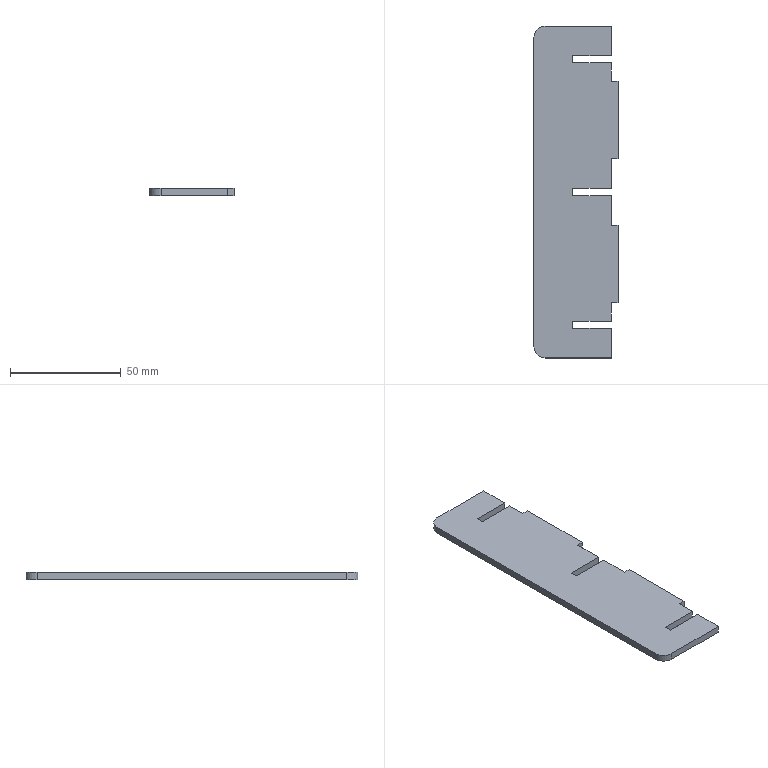Part | SolidWorks | features FlatPattern 1, SMBaseFlange 1, SheetMetal 1 | 1 solid | 28 faces | box 38 x 150 x 3.2 mm | volume 16900 mm3 | plane 26 | cylinder 2 | commonest cylinder face diameters 10 x2
STEP:
#1=CARTESIAN_POINT('',(-36.436,77.184,0.));
#2=VERTEX_POINT('',#1);
#3=CARTESIAN_POINT('',(-36.436,90.584,0.));
#4=VERTEX_POINT('',#3);
#5=CARTESIAN_POINT('',(-36.436,90.584,0.));
#6=DIRECTION('',(0.,1.,0.));
#7=VECTOR('',#6,1000.);
#8=LINE('',#5,#7);
#9=EDGE_CURVE('',#2,#4,#8,.T.);
#10=ORIENTED_EDGE('',*,*,#9,.F.);
#11=CARTESIAN_POINT('',(-36.436,77.184,-3.2));
#12=VERTEX_POINT('',#11);
#13=CARTESIAN_POINT('',(-36.436,77.184,-3.2));
#14=DIRECTION('',(0.,0.,1.));
#15=VECTOR('',#14,1000.);
#16=LINE('',#13,#15);
#17=EDGE_CURVE('',#12,#2,#16,.T.);
#18=ORIENTED_EDGE('',*,*,#17,.F.);
#19=CARTESIAN_POINT('',(-36.436,90.584,-3.2));
#20=VERTEX_POINT('',#19);
#21=CARTESIAN_POINT('',(-36.436,90.584,-3.2));
#22=DIRECTION('',(0.,1.,0.));
#23=VECTOR('',#22,1000.);
#24=LINE('',#21,#23);
#25=EDGE_CURVE('',#12,#20,#24,.T.);
#26=ORIENTED_EDGE('',*,*,#25,.T.);
#27=CARTESIAN_POINT('',(-36.436,90.584,-3.2));
#28=DIRECTION('',(0.,0.,1.));
#29=VECTOR('',#28,1000.);
#30=LINE('',#27,#29);
#31=EDGE_CURVE('',#20,#4,#30,.T.);
#32=ORIENTED_EDGE('',*,*,#31,.T.);
#33=EDGE_LOOP('',(#10,#18,#26,#32));
#34=FACE_OUTER_BOUND('',#33,.T.);
#35=CARTESIAN_POINT('',(-36.436,90.584,-3.2));
#36=DIRECTION('',(1.,0.,0.));
#37=DIRECTION('',(0.,1.,0.));
#38=AXIS2_PLACEMENT_3D('',#35,#36,#37);
#39=PLANE('',#38);
#40=ADVANCED_FACE('',(#34),#39,.T.);
#41=CARTESIAN_POINT('',(-53.936,77.184,0.));
#42=VERTEX_POINT('',#41);
#43=CARTESIAN_POINT('',(-36.436,77.184,0.));
#44=DIRECTION('',(1.,0.,0.));
#45=VECTOR('',#44,1000.);
#46=LINE('',#43,#45);
#47=EDGE_CURVE('',#42,#2,#46,.T.);
#48=ORIENTED_EDGE('',*,*,#47,.F.);
#49=CARTESIAN_POINT('',(-53.936,77.184,-3.2));
#50=VERTEX_POINT('',#49);
#51=CARTESIAN_POINT('',(-53.936,77.184,-3.2));
#52=DIRECTION('',(0.,0.,1.));
#53=VECTOR('',#52,1000.);
#54=LINE('',#51,#53);
#55=EDGE_CURVE('',#50,#42,#54,.T.);
#56=ORIENTED_EDGE('',*,*,#55,.F.);
#57=CARTESIAN_POINT('',(-36.436,77.184,-3.2));
#58=DIRECTION('',(1.,0.,0.));
#59=VECTOR('',#58,1000.);
#60=LINE('',#57,#59);
#61=EDGE_CURVE('',#50,#12,#60,.T.);
#62=ORIENTED_EDGE('',*,*,#61,.T.);
#63=ORIENTED_EDGE('',*,*,#17,.T.);
#64=EDGE_LOOP('',(#48,#56,#62,#63));
#65=FACE_OUTER_BOUND('',#64,.T.);
#66=CARTESIAN_POINT('',(-36.436,77.184,-3.2));
#67=DIRECTION('',(0.,-1.,0.));
#68=DIRECTION('',(0.,0.,-1.));
#69=AXIS2_PLACEMENT_3D('',#66,#67,#68);
#70=PLANE('',#69);
#71=ADVANCED_FACE('',(#65),#70,.T.);
#72=CARTESIAN_POINT('',(-53.936,73.984,0.));
#73=VERTEX_POINT('',#72);
#74=CARTESIAN_POINT('',(-53.936,77.184,0.));
#75=DIRECTION('',(0.,1.,0.));
#76=VECTOR('',#75,1000.);
#77=LINE('',#74,#76);
#78=EDGE_CURVE('',#73,#42,#77,.T.);
#79=ORIENTED_EDGE('',*,*,#78,.F.);
#80=CARTESIAN_POINT('',(-53.936,73.984,-3.2));
#81=VERTEX_POINT('',#80);
#82=CARTESIAN_POINT('',(-53.936,73.984,-3.2));
#83=DIRECTION('',(0.,0.,1.));
#84=VECTOR('',#83,1000.);
#85=LINE('',#82,#84);
#86=EDGE_CURVE('',#81,#73,#85,.T.);
#87=ORIENTED_EDGE('',*,*,#86,.F.);
#88=CARTESIAN_POINT('',(-53.936,77.184,-3.2));
#89=DIRECTION('',(0.,1.,0.));
#90=VECTOR('',#89,1000.);
#91=LINE('',#88,#90);
#92=EDGE_CURVE('',#81,#50,#91,.T.);
#93=ORIENTED_EDGE('',*,*,#92,.T.);
#94=ORIENTED_EDGE('',*,*,#55,.T.);
#95=EDGE_LOOP('',(#79,#87,#93,#94));
#96=FACE_OUTER_BOUND('',#95,.T.);
#97=CARTESIAN_POINT('',(-53.936,77.184,-3.2));
#98=DIRECTION('',(1.,0.,0.));
#99=DIRECTION('',(0.,0.,-1.));
#100=AXIS2_PLACEMENT_3D('',#97,#98,#99);
#101=PLANE('',#100);
#102=ADVANCED_FACE('',(#96),#101,.T.);
#103=CARTESIAN_POINT('',(-36.436,73.984,0.));
#104=VERTEX_POINT('',#103);
#105=CARTESIAN_POINT('',(-53.936,73.984,0.));
#106=DIRECTION('',(-1.,0.,0.));
#107=VECTOR('',#106,1000.);
#108=LINE('',#105,#107);
#109=EDGE_CURVE('',#104,#73,#108,.T.);
#110=ORIENTED_EDGE('',*,*,#109,.F.);
#111=CARTESIAN_POINT('',(-36.436,73.984,-3.2));
#112=VERTEX_POINT('',#111);
#113=CARTESIAN_POINT('',(-36.436,73.984,-3.2));
#114=DIRECTION('',(0.,0.,1.));
#115=VECTOR('',#114,1000.);
#116=LINE('',#113,#115);
#117=EDGE_CURVE('',#112,#104,#116,.T.);
#118=ORIENTED_EDGE('',*,*,#117,.F.);
#119=CARTESIAN_POINT('',(-53.936,73.984,-3.2));
#120=DIRECTION('',(-1.,0.,0.));
#121=VECTOR('',#120,1000.);
#122=LINE('',#119,#121);
#123=EDGE_CURVE('',#112,#81,#122,.T.);
#124=ORIENTED_EDGE('',*,*,#123,.T.);
#125=ORIENTED_EDGE('',*,*,#86,.T.);
#126=EDGE_LOOP('',(#110,#118,#124,#125));
#127=FACE_OUTER_BOUND('',#126,.T.);
#128=CARTESIAN_POINT('',(-53.936,73.984,-3.2));
#129=DIRECTION('',(0.,1.,0.));
#130=DIRECTION('',(0.,0.,1.));
#131=AXIS2_PLACEMENT_3D('',#128,#129,#130);
#132=PLANE('',#131);
#133=ADVANCED_FACE('',(#127),#132,.T.);
#134=CARTESIAN_POINT('',(-36.436,65.584,0.));
#135=VERTEX_POINT('',#134);
#136=CARTESIAN_POINT('',(-36.436,73.984,0.));
#137=DIRECTION('',(0.,1.,0.));
#138=VECTOR('',#137,1000.);
#139=LINE('',#136,#138);
#140=EDGE_CURVE('',#135,#104,#139,.T.);
#141=ORIENTED_EDGE('',*,*,#140,.F.);
#142=CARTESIAN_POINT('',(-36.436,65.584,-3.2));
#143=VERTEX_POINT('',#142);
#144=CARTESIAN_POINT('',(-36.436,65.584,-3.2));
#145=DIRECTION('',(0.,0.,1.));
#146=VECTOR('',#145,1000.);
#147=LINE('',#144,#146);
#148=EDGE_CURVE('',#143,#135,#147,.T.);
#149=ORIENTED_EDGE('',*,*,#148,.F.);
#150=CARTESIAN_POINT('',(-36.436,73.984,-3.2));
#151=DIRECTION('',(0.,1.,0.));
#152=VECTOR('',#151,1000.);
#153=LINE('',#150,#152);
#154=EDGE_CURVE('',#143,#112,#153,.T.);
#155=ORIENTED_EDGE('',*,*,#154,.T.);
#156=ORIENTED_EDGE('',*,*,#117,.T.);
#157=EDGE_LOOP('',(#141,#149,#155,#156));
#158=FACE_OUTER_BOUND('',#157,.T.);
#159=CARTESIAN_POINT('',(-36.436,73.984,-3.2));
#160=DIRECTION('',(1.,0.,0.));
#161=DIRECTION('',(0.,1.,0.));
#162=AXIS2_PLACEMENT_3D('',#159,#160,#161);
#163=PLANE('',#162);
#164=ADVANCED_FACE('',(#158),#163,.T.);
#165=CARTESIAN_POINT('',(-33.436,65.584,0.));
#166=VERTEX_POINT('',#165);
#167=CARTESIAN_POINT('',(-36.436,65.584,0.));
#168=DIRECTION('',(-1.,0.,0.));
#169=VECTOR('',#168,1000.);
#170=LINE('',#167,#169);
#171=EDGE_CURVE('',#166,#135,#170,.T.);
#172=ORIENTED_EDGE('',*,*,#171,.F.);
#173=CARTESIAN_POINT('',(-33.436,65.584,-3.2));
#174=VERTEX_POINT('',#173);
#175=CARTESIAN_POINT('',(-33.436,65.584,-3.2));
#176=DIRECTION('',(0.,0.,1.));
#177=VECTOR('',#176,1000.);
#178=LINE('',#175,#177);
#179=EDGE_CURVE('',#174,#166,#178,.T.);
#180=ORIENTED_EDGE('',*,*,#179,.F.);
#181=CARTESIAN_POINT('',(-36.436,65.584,-3.2));
#182=DIRECTION('',(-1.,0.,0.));
#183=VECTOR('',#182,1000.);
#184=LINE('',#181,#183);
#185=EDGE_CURVE('',#174,#143,#184,.T.);
#186=ORIENTED_EDGE('',*,*,#185,.T.);
#187=ORIENTED_EDGE('',*,*,#148,.T.);
#188=EDGE_LOOP('',(#172,#180,#186,#187));
#189=FACE_OUTER_BOUND('',#188,.T.);
#190=CARTESIAN_POINT('',(-36.436,65.584,-3.2));
#191=DIRECTION('',(0.,1.,0.));
#192=DIRECTION('',(0.,0.,1.));
#193=AXIS2_PLACEMENT_3D('',#190,#191,#192);
#194=PLANE('',#193);
#195=ADVANCED_FACE('',(#189),#194,.T.);
#196=CARTESIAN_POINT('',(-33.436,30.584,0.));
#197=VERTEX_POINT('',#196);
#198=CARTESIAN_POINT('',(-33.436,65.584,0.));
#199=DIRECTION('',(0.,1.,0.));
#200=VECTOR('',#199,1000.);
#201=LINE('',#198,#200);
#202=EDGE_CURVE('',#197,#166,#201,.T.);
#203=ORIENTED_EDGE('',*,*,#202,.F.);
#204=CARTESIAN_POINT('',(-33.436,30.584,-3.2));
#205=VERTEX_POINT('',#204);
#206=CARTESIAN_POINT('',(-33.436,30.584,-3.2));
#207=DIRECTION('',(0.,0.,1.));
#208=VECTOR('',#207,1000.);
#209=LINE('',#206,#208);
#210=EDGE_CURVE('',#205,#197,#209,.T.);
#211=ORIENTED_EDGE('',*,*,#210,.F.);
#212=CARTESIAN_POINT('',(-33.436,65.584,-3.2));
#213=DIRECTION('',(0.,1.,0.));
#214=VECTOR('',#213,1000.);
#215=LINE('',#212,#214);
#216=EDGE_CURVE('',#205,#174,#215,.T.);
#217=ORIENTED_EDGE('',*,*,#216,.T.);
#218=ORIENTED_EDGE('',*,*,#179,.T.);
#219=EDGE_LOOP('',(#203,#211,#217,#218));
#220=FACE_OUTER_BOUND('',#219,.T.);
#221=CARTESIAN_POINT('',(-33.436,65.584,-3.2));
#222=DIRECTION('',(1.,0.,0.));
#223=DIRECTION('',(0.,1.,0.));
#224=AXIS2_PLACEMENT_3D('',#221,#222,#223);
#225=PLANE('',#224);
#226=ADVANCED_FACE('',(#220),#225,.T.);
#227=CARTESIAN_POINT('',(-36.436,30.584,0.));
#228=VERTEX_POINT('',#227);
#229=CARTESIAN_POINT('',(-33.436,30.584,0.));
#230=DIRECTION('',(1.,0.,0.));
#231=VECTOR('',#230,1000.);
#232=LINE('',#229,#231);
#233=EDGE_CURVE('',#228,#197,#232,.T.);
#234=ORIENTED_EDGE('',*,*,#233,.F.);
#235=CARTESIAN_POINT('',(-36.436,30.584,-3.2));
#236=VERTEX_POINT('',#235);
#237=CARTESIAN_POINT('',(-36.436,30.584,-3.2));
#238=DIRECTION('',(0.,0.,1.));
#239=VECTOR('',#238,1000.);
#240=LINE('',#237,#239);
#241=EDGE_CURVE('',#236,#228,#240,.T.);
#242=ORIENTED_EDGE('',*,*,#241,.F.);
#243=CARTESIAN_POINT('',(-33.436,30.584,-3.2));
#244=DIRECTION('',(1.,0.,0.));
#245=VECTOR('',#244,1000.);
#246=LINE('',#243,#245);
#247=EDGE_CURVE('',#236,#205,#246,.T.);
#248=ORIENTED_EDGE('',*,*,#247,.T.);
#249=ORIENTED_EDGE('',*,*,#210,.T.);
#250=EDGE_LOOP('',(#234,#242,#248,#249));
#251=FACE_OUTER_BOUND('',#250,.T.);
#252=CARTESIAN_POINT('',(-33.436,30.584,-3.2));
#253=DIRECTION('',(0.,-1.,0.));
#254=DIRECTION('',(1.,0.,0.));
#255=AXIS2_PLACEMENT_3D('',#252,#253,#254);
#256=PLANE('',#255);
#257=ADVANCED_FACE('',(#251),#256,.T.);
#258=CARTESIAN_POINT('',(-36.436,17.184,0.));
#259=VERTEX_POINT('',#258);
#260=CARTESIAN_POINT('',(-36.436,30.584,0.));
#261=DIRECTION('',(0.,1.,0.));
#262=VECTOR('',#261,1000.);
#263=LINE('',#260,#262);
#264=EDGE_CURVE('',#259,#228,#263,.T.);
#265=ORIENTED_EDGE('',*,*,#264,.F.);
#266=CARTESIAN_POINT('',(-36.436,17.184,-3.2));
#267=VERTEX_POINT('',#266);
#268=CARTESIAN_POINT('',(-36.436,17.184,-3.2));
#269=DIRECTION('',(0.,0.,1.));
#270=VECTOR('',#269,1000.);
#271=LINE('',#268,#270);
#272=EDGE_CURVE('',#267,#259,#271,.T.);
#273=ORIENTED_EDGE('',*,*,#272,.F.);
#274=CARTESIAN_POINT('',(-36.436,30.584,-3.2));
#275=DIRECTION('',(0.,1.,0.));
#276=VECTOR('',#275,1000.);
#277=LINE('',#274,#276);
#278=EDGE_CURVE('',#267,#236,#277,.T.);
#279=ORIENTED_EDGE('',*,*,#278,.T.);
#280=ORIENTED_EDGE('',*,*,#241,.T.);
#281=EDGE_LOOP('',(#265,#273,#279,#280));
#282=FACE_OUTER_BOUND('',#281,.T.);
#283=CARTESIAN_POINT('',(-36.436,30.584,-3.2));
#284=DIRECTION('',(1.,0.,0.));
#285=DIRECTION('',(0.,1.,0.));
#286=AXIS2_PLACEMENT_3D('',#283,#284,#285);
#287=PLANE('',#286);
#288=ADVANCED_FACE('',(#282),#287,.T.);
#289=CARTESIAN_POINT('',(-53.936,17.184,0.));
#290=VERTEX_POINT('',#289);
#291=CARTESIAN_POINT('',(-36.436,17.184,0.));
#292=DIRECTION('',(1.,0.,0.));
#293=VECTOR('',#292,1000.);
#294=LINE('',#291,#293);
#295=EDGE_CURVE('',#290,#259,#294,.T.);
#296=ORIENTED_EDGE('',*,*,#295,.F.);
#297=CARTESIAN_POINT('',(-53.936,17.184,-3.2));
#298=VERTEX_POINT('',#297);
#299=CARTESIAN_POINT('',(-53.936,17.184,-3.2));
#300=DIRECTION('',(0.,0.,1.));
#301=VECTOR('',#300,1000.);
#302=LINE('',#299,#301);
#303=EDGE_CURVE('',#298,#290,#302,.T.);
#304=ORIENTED_EDGE('',*,*,#303,.F.);
#305=CARTESIAN_POINT('',(-36.436,17.184,-3.2));
#306=DIRECTION('',(1.,0.,0.));
#307=VECTOR('',#306,1000.);
#308=LINE('',#305,#307);
#309=EDGE_CURVE('',#298,#267,#308,.T.);
#310=ORIENTED_EDGE('',*,*,#309,.T.);
#311=ORIENTED_EDGE('',*,*,#272,.T.);
#312=EDGE_LOOP('',(#296,#304,#310,#311));
#313=FACE_OUTER_BOUND('',#312,.T.);
#314=CARTESIAN_POINT('',(-36.436,17.184,-3.2));
#315=DIRECTION('',(0.,-1.,0.));
#316=DIRECTION('',(0.,0.,-1.));
#317=AXIS2_PLACEMENT_3D('',#314,#315,#316);
#318=PLANE('',#317);
#319=ADVANCED_FACE('',(#313),#318,.T.);
#320=CARTESIAN_POINT('',(-53.936,13.984,0.));
#321=VERTEX_POINT('',#320);
#322=CARTESIAN_POINT('',(-53.936,17.184,0.));
#323=DIRECTION('',(0.,1.,0.));
#324=VECTOR('',#323,1000.);
#325=LINE('',#322,#324);
#326=EDGE_CURVE('',#321,#290,#325,.T.);
#327=ORIENTED_EDGE('',*,*,#326,.F.);
#328=CARTESIAN_POINT('',(-53.936,13.984,-3.2));
#329=VERTEX_POINT('',#328);
#330=CARTESIAN_POINT('',(-53.936,13.984,-3.2));
#331=DIRECTION('',(0.,0.,1.));
#332=VECTOR('',#331,1000.);
#333=LINE('',#330,#332);
#334=EDGE_CURVE('',#329,#321,#333,.T.);
#335=ORIENTED_EDGE('',*,*,#334,.F.);
#336=CARTESIAN_POINT('',(-53.936,17.184,-3.2));
#337=DIRECTION('',(0.,1.,0.));
#338=VECTOR('',#337,1000.);
#339=LINE('',#336,#338);
#340=EDGE_CURVE('',#329,#298,#339,.T.);
#341=ORIENTED_EDGE('',*,*,#340,.T.);
#342=ORIENTED_EDGE('',*,*,#303,.T.);
#343=EDGE_LOOP('',(#327,#335,#341,#342));
#344=FACE_OUTER_BOUND('',#343,.T.);
#345=CARTESIAN_POINT('',(-53.936,17.184,-3.2));
#346=DIRECTION('',(1.,0.,0.));
#347=DIRECTION('',(0.,0.,-1.));
#348=AXIS2_PLACEMENT_3D('',#345,#346,#347);
#349=PLANE('',#348);
#350=ADVANCED_FACE('',(#344),#349,.T.);
#351=CARTESIAN_POINT('',(-36.436,13.984,0.));
#352=VERTEX_POINT('',#351);
#353=CARTESIAN_POINT('',(-53.936,13.984,0.));
#354=DIRECTION('',(-1.,0.,0.));
#355=VECTOR('',#354,1000.);
#356=LINE('',#353,#355);
#357=EDGE_CURVE('',#352,#321,#356,.T.);
#358=ORIENTED_EDGE('',*,*,#357,.F.);
#359=CARTESIAN_POINT('',(-36.436,13.984,-3.2));
#360=VERTEX_POINT('',#359);
#361=CARTESIAN_POINT('',(-36.436,13.984,-3.2));
#362=DIRECTION('',(0.,0.,1.));
#363=VECTOR('',#362,1000.);
#364=LINE('',#361,#363);
#365=EDGE_CURVE('',#360,#352,#364,.T.);
#366=ORIENTED_EDGE('',*,*,#365,.F.);
#367=CARTESIAN_POINT('',(-53.936,13.984,-3.2));
#368=DIRECTION('',(-1.,0.,0.));
#369=VECTOR('',#368,1000.);
#370=LINE('',#367,#369);
#371=EDGE_CURVE('',#360,#329,#370,.T.);
#372=ORIENTED_EDGE('',*,*,#371,.T.);
#373=ORIENTED_EDGE('',*,*,#334,.T.);
#374=EDGE_LOOP('',(#358,#366,#372,#373));
#375=FACE_OUTER_BOUND('',#374,.T.);
#376=CARTESIAN_POINT('',(-53.936,13.984,-3.2));
#377=DIRECTION('',(0.,1.,0.));
#378=DIRECTION('',(0.,0.,1.));
#379=AXIS2_PLACEMENT_3D('',#376,#377,#378);
#380=PLANE('',#379);
#381=ADVANCED_FACE('',(#375),#380,.T.);
#382=CARTESIAN_POINT('',(-36.436,0.5843,0.));
#383=VERTEX_POINT('',#382);
#384=CARTESIAN_POINT('',(-36.436,13.984,0.));
#385=DIRECTION('',(0.,1.,0.));
#386=VECTOR('',#385,1000.);
#387=LINE('',#384,#386);
#388=EDGE_CURVE('',#383,#352,#387,.T.);
#389=ORIENTED_EDGE('',*,*,#388,.F.);
#390=CARTESIAN_POINT('',(-36.436,0.5843,-3.2));
#391=VERTEX_POINT('',#390);
#392=CARTESIAN_POINT('',(-36.436,0.5843,-3.2));
#393=DIRECTION('',(0.,0.,1.));
#394=VECTOR('',#393,1000.);
#395=LINE('',#392,#394);
#396=EDGE_CURVE('',#391,#383,#395,.T.);
#397=ORIENTED_EDGE('',*,*,#396,.F.);
#398=CARTESIAN_POINT('',(-36.436,13.984,-3.2));
#399=DIRECTION('',(0.,1.,0.));
#400=VECTOR('',#399,1000.);
#401=LINE('',#398,#400);
#402=EDGE_CURVE('',#391,#360,#401,.T.);
#403=ORIENTED_EDGE('',*,*,#402,.T.);
#404=ORIENTED_EDGE('',*,*,#365,.T.);
#405=EDGE_LOOP('',(#389,#397,#403,#404));
#406=FACE_OUTER_BOUND('',#405,.T.);
#407=CARTESIAN_POINT('',(-36.436,13.984,-3.2));
#408=DIRECTION('',(1.,0.,0.));
#409=DIRECTION('',(0.,1.,0.));
#410=AXIS2_PLACEMENT_3D('',#407,#408,#409);
#411=PLANE('',#410);
#412=ADVANCED_FACE('',(#406),#411,.T.);
#413=CARTESIAN_POINT('',(-33.436,0.5843,0.));
#414=VERTEX_POINT('',#413);
#415=CARTESIAN_POINT('',(-36.436,0.5843,0.));
#416=DIRECTION('',(-1.,0.,0.));
#417=VECTOR('',#416,1000.);
#418=LINE('',#415,#417);
#419=EDGE_CURVE('',#414,#383,#418,.T.);
#420=ORIENTED_EDGE('',*,*,#419,.F.);
#421=CARTESIAN_POINT('',(-33.436,0.5843,-3.2));
#422=VERTEX_POINT('',#421);
#423=CARTESIAN_POINT('',(-33.436,0.5843,-3.2));
#424=DIRECTION('',(0.,0.,1.));
#425=VECTOR('',#424,1000.);
#426=LINE('',#423,#425);
#427=EDGE_CURVE('',#422,#414,#426,.T.);
#428=ORIENTED_EDGE('',*,*,#427,.F.);
#429=CARTESIAN_POINT('',(-36.436,0.5843,-3.2));
#430=DIRECTION('',(-1.,0.,0.));
#431=VECTOR('',#430,1000.);
#432=LINE('',#429,#431);
#433=EDGE_CURVE('',#422,#391,#432,.T.);
#434=ORIENTED_EDGE('',*,*,#433,.T.);
#435=ORIENTED_EDGE('',*,*,#396,.T.);
#436=EDGE_LOOP('',(#420,#428,#434,#435));
#437=FACE_OUTER_BOUND('',#436,.T.);
#438=CARTESIAN_POINT('',(-36.436,0.5843,-3.2));
#439=DIRECTION('',(0.,1.,0.));
#440=DIRECTION('',(0.,0.,1.));
#441=AXIS2_PLACEMENT_3D('',#438,#439,#440);
#442=PLANE('',#441);
#443=ADVANCED_FACE('',(#437),#442,.T.);
#444=CARTESIAN_POINT('',(-33.436,-34.416,0.));
#445=VERTEX_POINT('',#444);
#446=CARTESIAN_POINT('',(-33.436,0.5843,0.));
#447=DIRECTION('',(0.,1.,0.));
#448=VECTOR('',#447,1000.);
#449=LINE('',#446,#448);
#450=EDGE_CURVE('',#445,#414,#449,.T.);
#451=ORIENTED_EDGE('',*,*,#450,.F.);
#452=CARTESIAN_POINT('',(-33.436,-34.416,-3.2));
#453=VERTEX_POINT('',#452);
#454=CARTESIAN_POINT('',(-33.436,-34.416,-3.2));
#455=DIRECTION('',(0.,0.,1.));
#456=VECTOR('',#455,1000.);
#457=LINE('',#454,#456);
#458=EDGE_CURVE('',#453,#445,#457,.T.);
#459=ORIENTED_EDGE('',*,*,#458,.F.);
#460=CARTESIAN_POINT('',(-33.436,0.5843,-3.2));
#461=DIRECTION('',(0.,1.,0.));
#462=VECTOR('',#461,1000.);
#463=LINE('',#460,#462);
#464=EDGE_CURVE('',#453,#422,#463,.T.);
#465=ORIENTED_EDGE('',*,*,#464,.T.);
#466=ORIENTED_EDGE('',*,*,#427,.T.);
#467=EDGE_LOOP('',(#451,#459,#465,#466));
#468=FACE_OUTER_BOUND('',#467,.T.);
#469=CARTESIAN_POINT('',(-33.436,0.5843,-3.2));
#470=DIRECTION('',(1.,0.,0.));
#471=DIRECTION('',(0.,1.,0.));
#472=AXIS2_PLACEMENT_3D('',#469,#470,#471);
#473=PLANE('',#472);
#474=ADVANCED_FACE('',(#468),#473,.T.);
#475=CARTESIAN_POINT('',(-36.436,-34.416,0.));
#476=VERTEX_POINT('',#475);
#477=CARTESIAN_POINT('',(-33.436,-34.416,0.));
#478=DIRECTION('',(1.,0.,0.));
#479=VECTOR('',#478,1000.);
#480=LINE('',#477,#479);
#481=EDGE_CURVE('',#476,#445,#480,.T.);
#482=ORIENTED_EDGE('',*,*,#481,.F.);
#483=CARTESIAN_POINT('',(-36.436,-34.416,-3.2));
#484=VERTEX_POINT('',#483);
#485=CARTESIAN_POINT('',(-36.436,-34.416,-3.2));
#486=DIRECTION('',(0.,0.,1.));
#487=VECTOR('',#486,1000.);
#488=LINE('',#485,#487);
#489=EDGE_CURVE('',#484,#476,#488,.T.);
#490=ORIENTED_EDGE('',*,*,#489,.F.);
#491=CARTESIAN_POINT('',(-33.436,-34.416,-3.2));
#492=DIRECTION('',(1.,0.,0.));
#493=VECTOR('',#492,1000.);
#494=LINE('',#491,#493);
#495=EDGE_CURVE('',#484,#453,#494,.T.);
#496=ORIENTED_EDGE('',*,*,#495,.T.);
#497=ORIENTED_EDGE('',*,*,#458,.T.);
#498=EDGE_LOOP('',(#482,#490,#496,#497));
#499=FACE_OUTER_BOUND('',#498,.T.);
#500=CARTESIAN_POINT('',(-33.436,-34.416,-3.2));
#501=DIRECTION('',(0.,-1.,0.));
#502=DIRECTION('',(1.,0.,0.));
#503=AXIS2_PLACEMENT_3D('',#500,#501,#502);
#504=PLANE('',#503);
#505=ADVANCED_FACE('',(#499),#504,.T.);
#506=CARTESIAN_POINT('',(-36.436,-42.816,0.));
#507=VERTEX_POINT('',#506);
#508=CARTESIAN_POINT('',(-36.436,-34.416,0.));
#509=DIRECTION('',(0.,1.,0.));
#510=VECTOR('',#509,1000.);
#511=LINE('',#508,#510);
#512=EDGE_CURVE('',#507,#476,#511,.T.);
#513=ORIENTED_EDGE('',*,*,#512,.F.);
#514=CARTESIAN_POINT('',(-36.436,-42.816,-3.2));
#515=VERTEX_POINT('',#514);
#516=CARTESIAN_POINT('',(-36.436,-42.816,-3.2));
#517=DIRECTION('',(0.,0.,1.));
#518=VECTOR('',#517,1000.);
#519=LINE('',#516,#518);
#520=EDGE_CURVE('',#515,#507,#519,.T.);
#521=ORIENTED_EDGE('',*,*,#520,.F.);
#522=CARTESIAN_POINT('',(-36.436,-34.416,-3.2));
#523=DIRECTION('',(0.,1.,0.));
#524=VECTOR('',#523,1000.);
#525=LINE('',#522,#524);
#526=EDGE_CURVE('',#515,#484,#525,.T.);
#527=ORIENTED_EDGE('',*,*,#526,.T.);
#528=ORIENTED_EDGE('',*,*,#489,.T.);
#529=EDGE_LOOP('',(#513,#521,#527,#528));
#530=FACE_OUTER_BOUND('',#529,.T.);
#531=CARTESIAN_POINT('',(-36.436,-34.416,-3.2));
#532=DIRECTION('',(1.,0.,0.));
#533=DIRECTION('',(0.,1.,0.));
#534=AXIS2_PLACEMENT_3D('',#531,#532,#533);
#535=PLANE('',#534);
#536=ADVANCED_FACE('',(#530),#535,.T.);
#537=CARTESIAN_POINT('',(-53.936,-42.816,0.));
#538=VERTEX_POINT('',#537);
#539=CARTESIAN_POINT('',(-36.436,-42.816,0.));
#540=DIRECTION('',(1.,0.,0.));
#541=VECTOR('',#540,1000.);
#542=LINE('',#539,#541);
#543=EDGE_CURVE('',#538,#507,#542,.T.);
#544=ORIENTED_EDGE('',*,*,#543,.F.);
#545=CARTESIAN_POINT('',(-53.936,-42.816,-3.2));
#546=VERTEX_POINT('',#545);
#547=CARTESIAN_POINT('',(-53.936,-42.816,-3.2));
#548=DIRECTION('',(0.,0.,1.));
#549=VECTOR('',#548,1000.);
#550=LINE('',#547,#549);
#551=EDGE_CURVE('',#546,#538,#550,.T.);
#552=ORIENTED_EDGE('',*,*,#551,.F.);
#553=CARTESIAN_POINT('',(-36.436,-42.816,-3.2));
#554=DIRECTION('',(1.,0.,0.));
#555=VECTOR('',#554,1000.);
#556=LINE('',#553,#555);
#557=EDGE_CURVE('',#546,#515,#556,.T.);
#558=ORIENTED_EDGE('',*,*,#557,.T.);
#559=ORIENTED_EDGE('',*,*,#520,.T.);
#560=EDGE_LOOP('',(#544,#552,#558,#559));
#561=FACE_OUTER_BOUND('',#560,.T.);
#562=CARTESIAN_POINT('',(-36.436,-42.816,-3.2));
#563=DIRECTION('',(0.,-1.,0.));
#564=DIRECTION('',(1.,0.,0.));
#565=AXIS2_PLACEMENT_3D('',#562,#563,#564);
#566=PLANE('',#565);
#567=ADVANCED_FACE('',(#561),#566,.T.);
#568=CARTESIAN_POINT('',(-53.936,-46.016,0.));
#569=VERTEX_POINT('',#568);
#570=CARTESIAN_POINT('',(-53.936,-42.816,0.));
#571=DIRECTION('',(0.,1.,0.));
#572=VECTOR('',#571,1000.);
#573=LINE('',#570,#572);
#574=EDGE_CURVE('',#569,#538,#573,.T.);
#575=ORIENTED_EDGE('',*,*,#574,.F.);
#576=CARTESIAN_POINT('',(-53.936,-46.016,-3.2));
#577=VERTEX_POINT('',#576);
#578=CARTESIAN_POINT('',(-53.936,-46.016,-3.2));
#579=DIRECTION('',(0.,0.,1.));
#580=VECTOR('',#579,1000.);
#581=LINE('',#578,#580);
#582=EDGE_CURVE('',#577,#569,#581,.T.);
#583=ORIENTED_EDGE('',*,*,#582,.F.);
#584=CARTESIAN_POINT('',(-53.936,-42.816,-3.2));
#585=DIRECTION('',(0.,1.,0.));
#586=VECTOR('',#585,1000.);
#587=LINE('',#584,#586);
#588=EDGE_CURVE('',#577,#546,#587,.T.);
#589=ORIENTED_EDGE('',*,*,#588,.T.);
#590=ORIENTED_EDGE('',*,*,#551,.T.);
#591=EDGE_LOOP('',(#575,#583,#589,#590));
#592=FACE_OUTER_BOUND('',#591,.T.);
#593=CARTESIAN_POINT('',(-53.936,-42.816,-3.2));
#594=DIRECTION('',(1.,0.,0.));
#595=DIRECTION('',(0.,0.,-1.));
#596=AXIS2_PLACEMENT_3D('',#593,#594,#595);
#597=PLANE('',#596);
#598=ADVANCED_FACE('',(#592),#597,.T.);
#599=CARTESIAN_POINT('',(-36.436,-46.016,0.));
#600=VERTEX_POINT('',#599);
#601=CARTESIAN_POINT('',(-53.936,-46.016,0.));
#602=DIRECTION('',(-1.,0.,0.));
#603=VECTOR('',#602,1000.);
#604=LINE('',#601,#603);
#605=EDGE_CURVE('',#600,#569,#604,.T.);
#606=ORIENTED_EDGE('',*,*,#605,.F.);
#607=CARTESIAN_POINT('',(-36.436,-46.016,-3.2));
#608=VERTEX_POINT('',#607);
#609=CARTESIAN_POINT('',(-36.436,-46.016,-3.2));
#610=DIRECTION('',(0.,0.,1.));
#611=VECTOR('',#610,1000.);
#612=LINE('',#609,#611);
#613=EDGE_CURVE('',#608,#600,#612,.T.);
#614=ORIENTED_EDGE('',*,*,#613,.F.);
#615=CARTESIAN_POINT('',(-53.936,-46.016,-3.2));
#616=DIRECTION('',(-1.,0.,0.));
#617=VECTOR('',#616,1000.);
#618=LINE('',#615,#617);
#619=EDGE_CURVE('',#608,#577,#618,.T.);
#620=ORIENTED_EDGE('',*,*,#619,.T.);
#621=ORIENTED_EDGE('',*,*,#582,.T.);
#622=EDGE_LOOP('',(#606,#614,#620,#621));
#623=FACE_OUTER_BOUND('',#622,.T.);
#624=CARTESIAN_POINT('',(-53.936,-46.016,-3.2));
#625=DIRECTION('',(0.,1.,0.));
#626=DIRECTION('',(-1.,0.,0.));
#627=AXIS2_PLACEMENT_3D('',#624,#625,#626);
#628=PLANE('',#627);
#629=ADVANCED_FACE('',(#623),#628,.T.);
#630=CARTESIAN_POINT('',(-36.436,-59.416,0.));
#631=VERTEX_POINT('',#630);
#632=CARTESIAN_POINT('',(-36.436,-46.016,0.));
#633=DIRECTION('',(0.,1.,0.));
#634=VECTOR('',#633,1000.);
#635=LINE('',#632,#634);
#636=EDGE_CURVE('',#631,#600,#635,.T.);
#637=ORIENTED_EDGE('',*,*,#636,.F.);
#638=CARTESIAN_POINT('',(-36.436,-59.416,-3.2));
#639=VERTEX_POINT('',#638);
#640=CARTESIAN_POINT('',(-36.436,-59.416,-3.2));
#641=DIRECTION('',(0.,0.,1.));
#642=VECTOR('',#641,1000.);
#643=LINE('',#640,#642);
#644=EDGE_CURVE('',#639,#631,#643,.T.);
#645=ORIENTED_EDGE('',*,*,#644,.F.);
#646=CARTESIAN_POINT('',(-36.436,-46.016,-3.2));
#647=DIRECTION('',(0.,1.,0.));
#648=VECTOR('',#647,1000.);
#649=LINE('',#646,#648);
#650=EDGE_CURVE('',#639,#608,#649,.T.);
#651=ORIENTED_EDGE('',*,*,#650,.T.);
#652=ORIENTED_EDGE('',*,*,#613,.T.);
#653=EDGE_LOOP('',(#637,#645,#651,#652));
#654=FACE_OUTER_BOUND('',#653,.T.);
#655=CARTESIAN_POINT('',(-36.436,-46.016,-3.2));
#656=DIRECTION('',(1.,0.,0.));
#657=DIRECTION('',(0.,1.,0.));
#658=AXIS2_PLACEMENT_3D('',#655,#656,#657);
#659=PLANE('',#658);
#660=ADVANCED_FACE('',(#654),#659,.T.);
#661=CARTESIAN_POINT('',(-66.436,-59.416,0.));
#662=VERTEX_POINT('',#661);
#663=CARTESIAN_POINT('',(-36.436,-59.416,0.));
#664=DIRECTION('',(1.,0.,0.));
#665=VECTOR('',#664,1000.);
#666=LINE('',#663,#665);
#667=EDGE_CURVE('',#662,#631,#666,.T.);
#668=ORIENTED_EDGE('',*,*,#667,.F.);
#669=CARTESIAN_POINT('',(-66.436,-59.416,-3.2));
#670=VERTEX_POINT('',#669);
#671=CARTESIAN_POINT('',(-66.436,-59.416,-3.2));
#672=DIRECTION('',(0.,0.,1.));
#673=VECTOR('',#672,1000.);
#674=LINE('',#671,#673);
#675=EDGE_CURVE('',#670,#662,#674,.T.);
#676=ORIENTED_EDGE('',*,*,#675,.F.);
#677=CARTESIAN_POINT('',(-36.436,-59.416,-3.2));
#678=DIRECTION('',(1.,0.,0.));
#679=VECTOR('',#678,1000.);
#680=LINE('',#677,#679);
#681=EDGE_CURVE('',#670,#639,#680,.T.);
#682=ORIENTED_EDGE('',*,*,#681,.T.);
#683=ORIENTED_EDGE('',*,*,#644,.T.);
#684=EDGE_LOOP('',(#668,#676,#682,#683));
#685=FACE_OUTER_BOUND('',#684,.T.);
#686=CARTESIAN_POINT('',(-36.436,-59.416,-3.2));
#687=DIRECTION('',(0.,-1.,0.));
#688=DIRECTION('',(1.,0.,0.));
#689=AXIS2_PLACEMENT_3D('',#686,#687,#688);
#690=PLANE('',#689);
#691=ADVANCED_FACE('',(#685),#690,.T.);
#692=CARTESIAN_POINT('',(-71.436,-54.416,0.));
#693=VERTEX_POINT('',#692);
#694=CARTESIAN_POINT('',(-66.436,-54.416,0.));
#695=DIRECTION('',(0.,0.,1.));
#696=DIRECTION('',(-1.,0.,0.));
#697=AXIS2_PLACEMENT_3D('',#694,#695,#696);
#698=CIRCLE('',#697,5.);
#699=EDGE_CURVE('',#693,#662,#698,.T.);
#700=ORIENTED_EDGE('',*,*,#699,.F.);
#701=CARTESIAN_POINT('',(-71.436,-54.416,-3.2));
#702=VERTEX_POINT('',#701);
#703=CARTESIAN_POINT('',(-71.436,-54.416,-3.2));
#704=DIRECTION('',(0.,0.,1.));
#705=VECTOR('',#704,1000.);
#706=LINE('',#703,#705);
#707=EDGE_CURVE('',#702,#693,#706,.T.);
#708=ORIENTED_EDGE('',*,*,#707,.F.);
#709=CARTESIAN_POINT('',(-66.436,-54.416,-3.2));
#710=DIRECTION('',(0.,0.,1.));
#711=DIRECTION('',(-1.,0.,0.));
#712=AXIS2_PLACEMENT_3D('',#709,#710,#711);
#713=CIRCLE('',#712,5.);
#714=EDGE_CURVE('',#702,#670,#713,.T.);
#715=ORIENTED_EDGE('',*,*,#714,.T.);
#716=ORIENTED_EDGE('',*,*,#675,.T.);
#717=EDGE_LOOP('',(#700,#708,#715,#716));
#718=FACE_OUTER_BOUND('',#717,.T.);
#719=CARTESIAN_POINT('',(-66.436,-54.416,-3.2));
#720=DIRECTION('',(0.,0.,1.));
#721=DIRECTION('',(1.,0.,0.));
#722=AXIS2_PLACEMENT_3D('',#719,#720,#721);
#723=CYLINDRICAL_SURFACE('',#722,5.);
#724=ADVANCED_FACE('',(#718),#723,.T.);
#725=CARTESIAN_POINT('',(-71.436,85.584,0.));
#726=VERTEX_POINT('',#725);
#727=CARTESIAN_POINT('',(-71.436,85.584,0.));
#728=DIRECTION('',(0.,-1.,0.));
#729=VECTOR('',#728,1000.);
#730=LINE('',#727,#729);
#731=EDGE_CURVE('',#726,#693,#730,.T.);
#732=ORIENTED_EDGE('',*,*,#731,.F.);
#733=CARTESIAN_POINT('',(-71.436,85.584,-3.2));
#734=VERTEX_POINT('',#733);
#735=CARTESIAN_POINT('',(-71.436,85.584,-3.2));
#736=DIRECTION('',(0.,0.,1.));
#737=VECTOR('',#736,1000.);
#738=LINE('',#735,#737);
#739=EDGE_CURVE('',#734,#726,#738,.T.);
#740=ORIENTED_EDGE('',*,*,#739,.F.);
#741=CARTESIAN_POINT('',(-71.436,85.584,-3.2));
#742=DIRECTION('',(0.,-1.,0.));
#743=VECTOR('',#742,1000.);
#744=LINE('',#741,#743);
#745=EDGE_CURVE('',#734,#702,#744,.T.);
#746=ORIENTED_EDGE('',*,*,#745,.T.);
#747=ORIENTED_EDGE('',*,*,#707,.T.);
#748=EDGE_LOOP('',(#732,#740,#746,#747));
#749=FACE_OUTER_BOUND('',#748,.T.);
#750=CARTESIAN_POINT('',(-71.436,85.584,-3.2));
#751=DIRECTION('',(-1.,0.,0.));
#752=DIRECTION('',(0.,-1.,0.));
#753=AXIS2_PLACEMENT_3D('',#750,#751,#752);
#754=PLANE('',#753);
#755=ADVANCED_FACE('',(#749),#754,.T.);
#756=CARTESIAN_POINT('',(-66.436,90.584,0.));
#757=VERTEX_POINT('',#756);
#758=CARTESIAN_POINT('',(-66.436,85.584,0.));
#759=DIRECTION('',(0.,0.,1.));
#760=DIRECTION('',(1.,0.,0.));
#761=AXIS2_PLACEMENT_3D('',#758,#759,#760);
#762=CIRCLE('',#761,5.);
#763=EDGE_CURVE('',#757,#726,#762,.T.);
#764=ORIENTED_EDGE('',*,*,#763,.F.);
#765=CARTESIAN_POINT('',(-66.436,90.584,-3.2));
#766=VERTEX_POINT('',#765);
#767=CARTESIAN_POINT('',(-66.436,90.584,-3.2));
#768=DIRECTION('',(0.,0.,1.));
#769=VECTOR('',#768,1000.);
#770=LINE('',#767,#769);
#771=EDGE_CURVE('',#766,#757,#770,.T.);
#772=ORIENTED_EDGE('',*,*,#771,.F.);
#773=CARTESIAN_POINT('',(-66.436,85.584,-3.2));
#774=DIRECTION('',(0.,0.,1.));
#775=DIRECTION('',(1.,0.,0.));
#776=AXIS2_PLACEMENT_3D('',#773,#774,#775);
#777=CIRCLE('',#776,5.);
#778=EDGE_CURVE('',#766,#734,#777,.T.);
#779=ORIENTED_EDGE('',*,*,#778,.T.);
#780=ORIENTED_EDGE('',*,*,#739,.T.);
#781=EDGE_LOOP('',(#764,#772,#779,#780));
#782=FACE_OUTER_BOUND('',#781,.T.);
#783=CARTESIAN_POINT('',(-66.436,85.584,-3.2));
#784=DIRECTION('',(0.,0.,1.));
#785=DIRECTION('',(1.,0.,0.));
#786=AXIS2_PLACEMENT_3D('',#783,#784,#785);
#787=CYLINDRICAL_SURFACE('',#786,5.);
#788=ADVANCED_FACE('',(#782),#787,.T.);
#789=CARTESIAN_POINT('',(-36.436,90.584,0.));
#790=DIRECTION('',(-1.,0.,0.));
#791=VECTOR('',#790,1000.);
#792=LINE('',#789,#791);
#793=EDGE_CURVE('',#4,#757,#792,.T.);
#794=ORIENTED_EDGE('',*,*,#793,.F.);
#795=ORIENTED_EDGE('',*,*,#31,.F.);
#796=CARTESIAN_POINT('',(-36.436,90.584,-3.2));
#797=DIRECTION('',(-1.,0.,0.));
#798=VECTOR('',#797,1000.);
#799=LINE('',#796,#798);
#800=EDGE_CURVE('',#20,#766,#799,.T.);
#801=ORIENTED_EDGE('',*,*,#800,.T.);
#802=ORIENTED_EDGE('',*,*,#771,.T.);
#803=EDGE_LOOP('',(#794,#795,#801,#802));
#804=FACE_OUTER_BOUND('',#803,.T.);
#805=CARTESIAN_POINT('',(-36.436,90.584,-3.2));
#806=DIRECTION('',(0.,1.,0.));
#807=DIRECTION('',(0.,0.,1.));
#808=AXIS2_PLACEMENT_3D('',#805,#806,#807);
#809=PLANE('',#808);
#810=ADVANCED_FACE('',(#804),#809,.T.);
#811=ORIENTED_EDGE('',*,*,#25,.F.);
#812=ORIENTED_EDGE('',*,*,#61,.F.);
#813=ORIENTED_EDGE('',*,*,#92,.F.);
#814=ORIENTED_EDGE('',*,*,#123,.F.);
#815=ORIENTED_EDGE('',*,*,#154,.F.);
#816=ORIENTED_EDGE('',*,*,#185,.F.);
#817=ORIENTED_EDGE('',*,*,#216,.F.);
#818=ORIENTED_EDGE('',*,*,#247,.F.);
#819=ORIENTED_EDGE('',*,*,#278,.F.);
#820=ORIENTED_EDGE('',*,*,#309,.F.);
#821=ORIENTED_EDGE('',*,*,#340,.F.);
#822=ORIENTED_EDGE('',*,*,#371,.F.);
#823=ORIENTED_EDGE('',*,*,#402,.F.);
#824=ORIENTED_EDGE('',*,*,#433,.F.);
#825=ORIENTED_EDGE('',*,*,#464,.F.);
#826=ORIENTED_EDGE('',*,*,#495,.F.);
#827=ORIENTED_EDGE('',*,*,#526,.F.);
#828=ORIENTED_EDGE('',*,*,#557,.F.);
#829=ORIENTED_EDGE('',*,*,#588,.F.);
#830=ORIENTED_EDGE('',*,*,#619,.F.);
#831=ORIENTED_EDGE('',*,*,#650,.F.);
#832=ORIENTED_EDGE('',*,*,#681,.F.);
#833=ORIENTED_EDGE('',*,*,#714,.F.);
#834=ORIENTED_EDGE('',*,*,#745,.F.);
#835=ORIENTED_EDGE('',*,*,#778,.F.);
#836=ORIENTED_EDGE('',*,*,#800,.F.);
#837=EDGE_LOOP('',(#811,#812,#813,#814,#815,#816,#817,#818,#819,#820,#821,#822,#823,#824,#825,#826,#827,#828,#829,#830,#831,#832,#833,#834,#835,#836));
#838=FACE_OUTER_BOUND('',#837,.T.);
#839=CARTESIAN_POINT('',(-66.436,-54.416,-3.2));
#840=DIRECTION('',(0.,0.,-1.));
#841=DIRECTION('',(-1.,0.,0.));
#842=AXIS2_PLACEMENT_3D('',#839,#840,#841);
#843=PLANE('',#842);
#844=ADVANCED_FACE('',(#838),#843,.T.);
#845=ORIENTED_EDGE('',*,*,#9,.T.);
#846=ORIENTED_EDGE('',*,*,#793,.T.);
#847=ORIENTED_EDGE('',*,*,#763,.T.);
#848=ORIENTED_EDGE('',*,*,#731,.T.);
#849=ORIENTED_EDGE('',*,*,#699,.T.);
#850=ORIENTED_EDGE('',*,*,#667,.T.);
#851=ORIENTED_EDGE('',*,*,#636,.T.);
#852=ORIENTED_EDGE('',*,*,#605,.T.);
#853=ORIENTED_EDGE('',*,*,#574,.T.);
#854=ORIENTED_EDGE('',*,*,#543,.T.);
#855=ORIENTED_EDGE('',*,*,#512,.T.);
#856=ORIENTED_EDGE('',*,*,#481,.T.);
#857=ORIENTED_EDGE('',*,*,#450,.T.);
#858=ORIENTED_EDGE('',*,*,#419,.T.);
#859=ORIENTED_EDGE('',*,*,#388,.T.);
#860=ORIENTED_EDGE('',*,*,#357,.T.);
#861=ORIENTED_EDGE('',*,*,#326,.T.);
#862=ORIENTED_EDGE('',*,*,#295,.T.);
#863=ORIENTED_EDGE('',*,*,#264,.T.);
#864=ORIENTED_EDGE('',*,*,#233,.T.);
#865=ORIENTED_EDGE('',*,*,#202,.T.);
#866=ORIENTED_EDGE('',*,*,#171,.T.);
#867=ORIENTED_EDGE('',*,*,#140,.T.);
#868=ORIENTED_EDGE('',*,*,#109,.T.);
#869=ORIENTED_EDGE('',*,*,#78,.T.);
#870=ORIENTED_EDGE('',*,*,#47,.T.);
#871=EDGE_LOOP('',(#845,#846,#847,#848,#849,#850,#851,#852,#853,#854,#855,#856,#857,#858,#859,#860,#861,#862,#863,#864,#865,#866,#867,#868,#869,#870));
#872=FACE_OUTER_BOUND('',#871,.T.);
#873=CARTESIAN_POINT('',(-66.436,-54.416,0.));
#874=DIRECTION('',(0.,0.,-1.));
#875=DIRECTION('',(-1.,0.,0.));
#876=AXIS2_PLACEMENT_3D('',#873,#874,#875);
#877=PLANE('',#876);
#878=ADVANCED_FACE('',(#872),#877,.F.);
#879=CLOSED_SHELL('',(#40,#71,#102,#133,#164,#195,#226,#257,#288,#319,#350,#381,#412,#443,#474,#505,#536,#567,#598,#629,#660,#691,#724,#755,#788,#810,#844,#878));
#880=MANIFOLD_SOLID_BREP('',#879);
#881=CARTESIAN_POINT('',(0.,0.,0.));
#882=DIRECTION('',(0.,0.,1.));
#883=DIRECTION('',(1.,0.,0.));
#884=AXIS2_PLACEMENT_3D('',#881,#882,#883);
#885=(LENGTH_UNIT()NAMED_UNIT(*)SI_UNIT(.MILLI.,.METRE.));
#886=UNCERTAINTY_MEASURE_WITH_UNIT(LENGTH_MEASURE(0.00001),#885,'','');
#887=(NAMED_UNIT(*)PLANE_ANGLE_UNIT()SI_UNIT($,.RADIAN.));
#888=(NAMED_UNIT(*)SI_UNIT($,.STERADIAN.)SOLID_ANGLE_UNIT());
#889=(GEOMETRIC_REPRESENTATION_CONTEXT(3)GLOBAL_UNCERTAINTY_ASSIGNED_CONTEXT((#886))GLOBAL_UNIT_ASSIGNED_CONTEXT((#885,#887,#888))REPRESENTATION_CONTEXT('',''));
#890=ADVANCED_BREP_SHAPE_REPRESENTATION('',(#880,#884),#889);